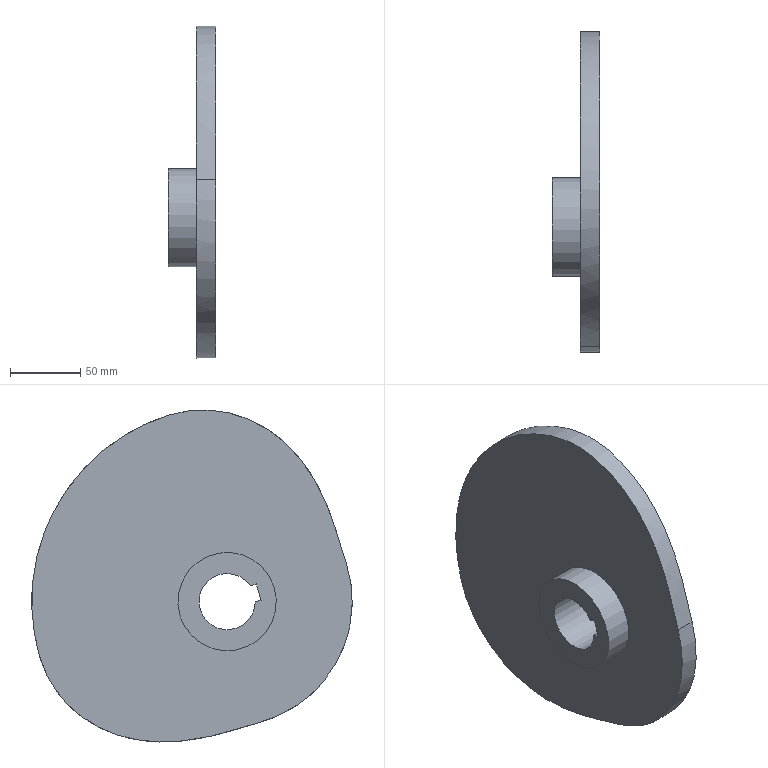Part | NX | features 100X000 2 | 1 solid | 10 faces | box 34 x 228.009 x 236.372 mm | volume 622668 mm3 | plane 6 | cylinder 2 | spline 2 | commonest cylinder face diameters 40 x1 70 x1
STEP:
#1=CARTESIAN_POINT('',(-103.5,-135.529,-808.87));
#2=VERTEX_POINT('',#1);
#3=CARTESIAN_POINT('',(-103.5,-138.999,-820.357));
#4=VERTEX_POINT('',#3);
#5=CARTESIAN_POINT('',(-103.5,-119.,-820.129));
#6=DIRECTION('',(-1.,0.,0.));
#7=DIRECTION('',(0.,0.9573,-0.2891));
#8=AXIS2_PLACEMENT_3D('',#5,#6,#7);
#9=CIRCLE('',#8,20.);
#10=EDGE_CURVE('',#2,#4,#9,.T.);
#11=ORIENTED_EDGE('',*,*,#10,.F.);
#12=CARTESIAN_POINT('',(-137.5,-135.529,-808.87));
#13=VERTEX_POINT('',#12);
#14=CARTESIAN_POINT('',(-103.5,-135.529,-808.87));
#15=DIRECTION('',(-1.,0.,0.));
#16=VECTOR('',#15,1000.);
#17=LINE('',#14,#16);
#18=EDGE_CURVE('',#2,#13,#17,.T.);
#19=ORIENTED_EDGE('',*,*,#18,.T.);
#20=CARTESIAN_POINT('',(-137.5,-138.999,-820.357));
#21=VERTEX_POINT('',#20);
#22=CARTESIAN_POINT('',(-137.5,-119.,-820.129));
#23=DIRECTION('',(1.,0.,0.));
#24=DIRECTION('',(0.,0.9573,-0.2891));
#25=AXIS2_PLACEMENT_3D('',#22,#23,#24);
#26=CIRCLE('',#25,20.);
#27=EDGE_CURVE('',#21,#13,#26,.T.);
#28=ORIENTED_EDGE('',*,*,#27,.F.);
#29=CARTESIAN_POINT('',(-137.5,-138.999,-820.357));
#30=DIRECTION('',(1.,0.,0.));
#31=VECTOR('',#30,1000.);
#32=LINE('',#29,#31);
#33=EDGE_CURVE('',#21,#4,#32,.T.);
#34=ORIENTED_EDGE('',*,*,#33,.T.);
#35=EDGE_LOOP('',(#11,#19,#28,#34));
#36=FACE_BOUND('',#35,.T.);
#37=CARTESIAN_POINT('',(218.943,-119.,-820.129));
#38=DIRECTION('',(-1.,0.,0.));
#39=DIRECTION('',(0.,0.9573,-0.2891));
#40=AXIS2_PLACEMENT_3D('',#37,#38,#39);
#41=CYLINDRICAL_SURFACE('',#40,20.);
#42=ADVANCED_FACE('',(#36),#41,.F.);
#43=CARTESIAN_POINT('',(-137.5,-143.231,-819.079));
#44=VERTEX_POINT('',#43);
#45=CARTESIAN_POINT('',(-137.5,-143.231,-819.079));
#46=DIRECTION('',(0.,0.9573,-0.2891));
#47=VECTOR('',#46,1000.);
#48=LINE('',#45,#47);
#49=EDGE_CURVE('',#44,#21,#48,.T.);
#50=ORIENTED_EDGE('',*,*,#49,.F.);
#51=CARTESIAN_POINT('',(-103.5,-143.231,-819.079));
#52=VERTEX_POINT('',#51);
#53=CARTESIAN_POINT('',(-137.5,-143.231,-819.079));
#54=DIRECTION('',(1.,0.,0.));
#55=VECTOR('',#54,1000.);
#56=LINE('',#53,#55);
#57=EDGE_CURVE('',#44,#52,#56,.T.);
#58=ORIENTED_EDGE('',*,*,#57,.T.);
#59=CARTESIAN_POINT('',(-103.5,-143.231,-819.079));
#60=DIRECTION('',(0.,0.9573,-0.2891));
#61=VECTOR('',#60,1000.);
#62=LINE('',#59,#61);
#63=EDGE_CURVE('',#52,#4,#62,.T.);
#64=ORIENTED_EDGE('',*,*,#63,.T.);
#65=ORIENTED_EDGE('',*,*,#33,.F.);
#66=EDGE_LOOP('',(#50,#58,#64,#65));
#67=FACE_BOUND('',#66,.T.);
#68=CARTESIAN_POINT('',(-103.5,-143.231,-819.079));
#69=DIRECTION('',(0.,-0.2891,-0.9573));
#70=DIRECTION('',(-1.,0.,0.));
#71=AXIS2_PLACEMENT_3D('',#68,#69,#70);
#72=PLANE('',#71);
#73=ADVANCED_FACE('',(#67),#72,.F.);
#74=CARTESIAN_POINT('',(-137.5,-139.762,-807.591));
#75=VERTEX_POINT('',#74);
#76=CARTESIAN_POINT('',(-137.5,-139.762,-807.591));
#77=DIRECTION('',(0.,-0.2891,-0.9573));
#78=VECTOR('',#77,1000.);
#79=LINE('',#76,#78);
#80=EDGE_CURVE('',#75,#44,#79,.T.);
#81=ORIENTED_EDGE('',*,*,#80,.F.);
#82=CARTESIAN_POINT('',(-103.5,-139.762,-807.591));
#83=VERTEX_POINT('',#82);
#84=CARTESIAN_POINT('',(-137.5,-139.762,-807.591));
#85=DIRECTION('',(1.,0.,0.));
#86=VECTOR('',#85,1000.);
#87=LINE('',#84,#86);
#88=EDGE_CURVE('',#75,#83,#87,.T.);
#89=ORIENTED_EDGE('',*,*,#88,.T.);
#90=CARTESIAN_POINT('',(-103.5,-139.762,-807.591));
#91=DIRECTION('',(0.,-0.2891,-0.9573));
#92=VECTOR('',#91,1000.);
#93=LINE('',#90,#92);
#94=EDGE_CURVE('',#83,#52,#93,.T.);
#95=ORIENTED_EDGE('',*,*,#94,.T.);
#96=ORIENTED_EDGE('',*,*,#57,.F.);
#97=EDGE_LOOP('',(#81,#89,#95,#96));
#98=FACE_BOUND('',#97,.T.);
#99=CARTESIAN_POINT('',(-103.5,-139.762,-807.591));
#100=DIRECTION('',(0.,-0.9573,0.2891));
#101=DIRECTION('',(-1.,0.,0.));
#102=AXIS2_PLACEMENT_3D('',#99,#100,#101);
#103=PLANE('',#102);
#104=ADVANCED_FACE('',(#98),#103,.F.);
#105=CARTESIAN_POINT('',(-117.5,-85.495,-830.249));
#106=VERTEX_POINT('',#105);
#107=CARTESIAN_POINT('',(-117.5,-119.,-820.129));
#108=DIRECTION('',(1.,0.,0.));
#109=DIRECTION('',(0.,0.9573,-0.2891));
#110=AXIS2_PLACEMENT_3D('',#107,#108,#109);
#111=CIRCLE('',#110,35.);
#112=EDGE_CURVE('',#106,#106,#111,.T.);
#113=ORIENTED_EDGE('',*,*,#112,.T.);
#114=EDGE_LOOP('',(#113));
#115=FACE_BOUND('',#114,.T.);
#116=CARTESIAN_POINT('',(-117.5,19.885,-825.794));
#117=VERTEX_POINT('',#116);
#118=CARTESIAN_POINT('',(-117.5,-203.83,-793.175));
#119=VERTEX_POINT('',#118);
#120=CARTESIAN_POINT('',(-117.5,-203.83,-793.175));
#121=CARTESIAN_POINT('',(-117.5,-206.1,-800.388));
#122=CARTESIAN_POINT('',(-117.5,-208.848,-815.383));
#123=CARTESIAN_POINT('',(-117.5,-207.135,-838.192));
#124=CARTESIAN_POINT('',(-117.5,-199.735,-859.831));
#125=CARTESIAN_POINT('',(-117.5,-187.117,-878.906));
#126=CARTESIAN_POINT('',(-117.5,-172.931,-891.635));
#127=CARTESIAN_POINT('',(-117.5,-159.935,-899.426));
#128=CARTESIAN_POINT('',(-117.5,-149.523,-903.996));
#129=CARTESIAN_POINT('',(-117.5,-138.618,-907.151));
#130=CARTESIAN_POINT('',(-117.5,-127.771,-910.449));
#131=CARTESIAN_POINT('',(-117.5,-116.863,-913.557));
#132=CARTESIAN_POINT('',(-117.5,-102.193,-917.232));
#133=CARTESIAN_POINT('',(-117.5,-83.496,-920.321));
#134=CARTESIAN_POINT('',(-117.5,-60.703,-920.128));
#135=CARTESIAN_POINT('',(-117.5,-38.429,-915.11));
#136=CARTESIAN_POINT('',(-117.5,-17.963,-904.903));
#137=CARTESIAN_POINT('',(-117.5,-0.8503,-889.705));
#138=CARTESIAN_POINT('',(-117.5,9.45,-873.606));
#139=CARTESIAN_POINT('',(-117.5,14.561,-859.339));
#140=CARTESIAN_POINT('',(-117.5,18.158,-844.637));
#141=CARTESIAN_POINT('',(-117.5,19.577,-833.35));
#142=CARTESIAN_POINT('',(-117.5,19.885,-825.794));
#143=B_SPLINE_CURVE_WITH_KNOTS('',3,(#120,#121,#122,#123,#124,#125,#126,#127,#128,#129,#130,#131,#132,#133,#134,#135,#136,#137,#138,#139,#140,#141,#142),.UNSPECIFIED.,.F.,.F.,(4,1,1,1,1,1,1,1,1,1,1,1,1,1,1,1,1,1,1,1,4),(0.,0.0625,0.125,0.1875,0.25,0.3125,0.3438,0.375,0.4062,0.4375,0.4688,0.5,0.5625,0.625,0.6875,0.75,0.8125,0.875,0.9062,0.9375,1.),.UNSPECIFIED.);
#144=EDGE_CURVE('',#117,#119,#143,.F.);
#145=ORIENTED_EDGE('',*,*,#144,.T.);
#146=CARTESIAN_POINT('',(-117.5,19.885,-825.794));
#147=CARTESIAN_POINT('',(-117.5,20.542,-810.441));
#148=CARTESIAN_POINT('',(-117.5,17.598,-787.258));
#149=CARTESIAN_POINT('',(-117.5,6.307,-758.571));
#150=CARTESIAN_POINT('',(-117.5,-5.545,-738.715));
#151=CARTESIAN_POINT('',(-117.5,-20.544,-721.111));
#152=CARTESIAN_POINT('',(-117.5,-38.233,-706.218));
#153=CARTESIAN_POINT('',(-117.5,-54.822,-696.403));
#154=CARTESIAN_POINT('',(-117.5,-68.935,-690.31));
#155=CARTESIAN_POINT('',(-117.5,-79.835,-686.529));
#156=CARTESIAN_POINT('',(-117.5,-91.128,-684.099));
#157=CARTESIAN_POINT('',(-117.5,-106.512,-683.184));
#158=CARTESIAN_POINT('',(-117.5,-125.675,-686.158));
#159=CARTESIAN_POINT('',(-117.5,-146.824,-695.82));
#160=CARTESIAN_POINT('',(-117.5,-164.847,-710.451));
#161=CARTESIAN_POINT('',(-117.5,-179.089,-728.734));
#162=CARTESIAN_POINT('',(-117.5,-189.587,-749.337));
#163=CARTESIAN_POINT('',(-117.5,-197.236,-771.098));
#164=CARTESIAN_POINT('',(-117.5,-201.598,-785.826));
#165=CARTESIAN_POINT('',(-117.5,-203.83,-793.175));
#166=B_SPLINE_CURVE_WITH_KNOTS('',3,(#146,#147,#148,#149,#150,#151,#152,#153,#154,#155,#156,#157,#158,#159,#160,#161,#162,#163,#164,#165),.UNSPECIFIED.,.F.,.F.,(4,1,1,1,1,1,1,1,1,1,1,1,1,1,1,1,1,4),(0.,0.125,0.1875,0.25,0.3125,0.375,0.4375,0.4688,0.5,0.5312,0.5625,0.625,0.6875,0.75,0.8125,0.875,0.9375,1.),.UNSPECIFIED.);
#167=EDGE_CURVE('',#119,#117,#166,.F.);
#168=ORIENTED_EDGE('',*,*,#167,.T.);
#169=EDGE_LOOP('',(#145,#168));
#170=FACE_BOUND('',#169,.T.);
#171=CARTESIAN_POINT('',(-117.5,-47.929,-928.307));
#172=DIRECTION('',(1.,0.,0.));
#173=DIRECTION('',(0.,-0.9573,0.2891));
#174=AXIS2_PLACEMENT_3D('',#171,#172,#173);
#175=PLANE('',#174);
#176=ADVANCED_FACE('',(#115,#170),#175,.F.);
#177=CARTESIAN_POINT('',(-103.5,-203.83,-793.175));
#178=VERTEX_POINT('',#177);
#179=CARTESIAN_POINT('',(-103.5,19.885,-825.794));
#180=VERTEX_POINT('',#179);
#181=CARTESIAN_POINT('',(-103.5,19.885,-825.794));
#182=CARTESIAN_POINT('',(-103.5,19.577,-833.349));
#183=CARTESIAN_POINT('',(-103.5,18.156,-844.636));
#184=CARTESIAN_POINT('',(-103.5,14.565,-859.339));
#185=CARTESIAN_POINT('',(-103.5,9.449,-873.606));
#186=CARTESIAN_POINT('',(-103.5,-0.8495,-889.704));
#187=CARTESIAN_POINT('',(-103.5,-17.962,-904.902));
#188=CARTESIAN_POINT('',(-103.5,-38.428,-915.11));
#189=CARTESIAN_POINT('',(-103.5,-60.702,-920.127));
#190=CARTESIAN_POINT('',(-103.5,-83.495,-920.321));
#191=CARTESIAN_POINT('',(-103.5,-102.191,-917.232));
#192=CARTESIAN_POINT('',(-103.5,-116.861,-913.557));
#193=CARTESIAN_POINT('',(-103.5,-127.77,-910.452));
#194=CARTESIAN_POINT('',(-103.5,-138.615,-907.15));
#195=CARTESIAN_POINT('',(-103.5,-149.521,-903.996));
#196=CARTESIAN_POINT('',(-103.5,-159.928,-899.413));
#197=CARTESIAN_POINT('',(-103.5,-172.931,-891.638));
#198=CARTESIAN_POINT('',(-103.5,-187.116,-878.904));
#199=CARTESIAN_POINT('',(-103.5,-199.733,-859.831));
#200=CARTESIAN_POINT('',(-103.5,-209.614,-830.978));
#201=CARTESIAN_POINT('',(-103.5,-208.416,-807.592));
#202=CARTESIAN_POINT('',(-103.5,-203.83,-793.175));
#203=B_SPLINE_CURVE_WITH_KNOTS('',3,(#181,#182,#183,#184,#185,#186,#187,#188,#189,#190,#191,#192,#193,#194,#195,#196,#197,#198,#199,#200,#201,#202),.UNSPECIFIED.,.F.,.F.,(4,1,1,1,1,1,1,1,1,1,1,1,1,1,1,1,1,1,1,4),(0.,0.0625,0.09375,0.125,0.1875,0.25,0.3125,0.375,0.4375,0.5,0.5312,0.5625,0.5938,0.625,0.6562,0.6875,0.75,0.8125,0.875,1.),.UNSPECIFIED.);
#204=EDGE_CURVE('',#178,#180,#203,.F.);
#205=ORIENTED_EDGE('',*,*,#204,.F.);
#206=CARTESIAN_POINT('',(-103.111,-203.83,-793.175));
#207=DIRECTION('',(-1.,0.,0.));
#208=VECTOR('',#207,1000.);
#209=LINE('',#206,#208);
#210=EDGE_CURVE('',#119,#178,#209,.F.);
#211=ORIENTED_EDGE('',*,*,#210,.F.);
#212=ORIENTED_EDGE('',*,*,#144,.F.);
#213=CARTESIAN_POINT('',(-103.111,19.885,-825.794));
#214=DIRECTION('',(-1.,0.,0.));
#215=VECTOR('',#214,1000.);
#216=LINE('',#213,#215);
#217=EDGE_CURVE('',#180,#117,#216,.T.);
#218=ORIENTED_EDGE('',*,*,#217,.F.);
#219=EDGE_LOOP('',(#205,#211,#212,#218));
#220=FACE_BOUND('',#219,.T.);
#221=CARTESIAN_POINT('',(-103.5,19.885,-825.794));
#222=CARTESIAN_POINT('',(-117.5,19.885,-825.794));
#223=CARTESIAN_POINT('',(-103.5,19.56,-833.741));
#224=CARTESIAN_POINT('',(-117.5,19.56,-833.741));
#225=CARTESIAN_POINT('',(-103.5,18.028,-845.325));
#226=CARTESIAN_POINT('',(-117.5,18.028,-845.325));
#227=CARTESIAN_POINT('',(-103.5,14.433,-859.739));
#228=CARTESIAN_POINT('',(-117.5,14.433,-859.739));
#229=CARTESIAN_POINT('',(-103.5,10.73,-869.978));
#230=CARTESIAN_POINT('',(-117.5,10.73,-869.978));
#231=CARTESIAN_POINT('',(-103.5,5.619,-879.516));
#232=CARTESIAN_POINT('',(-117.5,5.619,-879.516));
#233=CARTESIAN_POINT('',(-103.5,-0.8391,-888.445));
#234=CARTESIAN_POINT('',(-117.5,-0.8391,-888.445));
#235=CARTESIAN_POINT('',(-103.5,-8.305,-896.284));
#236=CARTESIAN_POINT('',(-117.5,-8.305,-896.284));
#237=CARTESIAN_POINT('',(-103.5,-16.795,-903.159));
#238=CARTESIAN_POINT('',(-117.5,-16.795,-903.159));
#239=CARTESIAN_POINT('',(-103.5,-26.109,-908.906));
#240=CARTESIAN_POINT('',(-117.5,-26.109,-908.906));
#241=CARTESIAN_POINT('',(-103.5,-35.953,-913.434));
#242=CARTESIAN_POINT('',(-117.5,-35.953,-913.434));
#243=CARTESIAN_POINT('',(-103.5,-46.394,-916.828));
#244=CARTESIAN_POINT('',(-117.5,-46.394,-916.828));
#245=CARTESIAN_POINT('',(-103.5,-57.036,-919.01));
#246=CARTESIAN_POINT('',(-117.5,-57.036,-919.01));
#247=CARTESIAN_POINT('',(-103.5,-67.843,-920.084));
#248=CARTESIAN_POINT('',(-117.5,-67.843,-920.084));
#249=CARTESIAN_POINT('',(-103.5,-82.467,-920.113));
#250=CARTESIAN_POINT('',(-117.5,-82.467,-920.113));
#251=CARTESIAN_POINT('',(-103.5,-96.728,-918.261));
#252=CARTESIAN_POINT('',(-117.5,-96.728,-918.261));
#253=CARTESIAN_POINT('',(-103.5,-110.806,-915.131));
#254=CARTESIAN_POINT('',(-117.5,-110.806,-915.131));
#255=CARTESIAN_POINT('',(-103.5,-121.295,-912.321));
#256=CARTESIAN_POINT('',(-117.5,-121.295,-912.321));
#257=CARTESIAN_POINT('',(-103.5,-131.724,-909.263));
#258=CARTESIAN_POINT('',(-117.5,-131.724,-909.263));
#259=CARTESIAN_POINT('',(-103.5,-140.397,-906.626));
#260=CARTESIAN_POINT('',(-117.5,-140.397,-906.626));
#261=CARTESIAN_POINT('',(-103.5,-147.324,-904.566));
#262=CARTESIAN_POINT('',(-117.5,-147.324,-904.566));
#263=CARTESIAN_POINT('',(-103.5,-154.26,-901.993));
#264=CARTESIAN_POINT('',(-117.5,-154.26,-901.993));
#265=CARTESIAN_POINT('',(-103.5,-162.89,-897.85));
#266=CARTESIAN_POINT('',(-117.5,-162.89,-897.85));
#267=CARTESIAN_POINT('',(-103.5,-172.887,-891.306));
#268=CARTESIAN_POINT('',(-117.5,-172.887,-891.306));
#269=CARTESIAN_POINT('',(-103.5,-185.273,-880.538));
#270=CARTESIAN_POINT('',(-117.5,-185.273,-880.538));
#271=CARTESIAN_POINT('',(-103.5,-198.112,-863.518));
#272=CARTESIAN_POINT('',(-117.5,-198.112,-863.518));
#273=CARTESIAN_POINT('',(-103.5,-207.077,-839.501));
#274=CARTESIAN_POINT('',(-117.5,-207.077,-839.501));
#275=CARTESIAN_POINT('',(-103.5,-208.585,-819.052));
#276=CARTESIAN_POINT('',(-117.5,-208.585,-819.052));
#277=CARTESIAN_POINT('',(-103.5,-206.738,-803.737));
#278=CARTESIAN_POINT('',(-117.5,-206.738,-803.737));
#279=CARTESIAN_POINT('',(-103.5,-204.877,-796.643));
#280=CARTESIAN_POINT('',(-117.5,-204.877,-796.643));
#281=CARTESIAN_POINT('',(-103.5,-203.83,-793.175));
#282=CARTESIAN_POINT('',(-117.5,-203.83,-793.175));
#283=B_SPLINE_SURFACE_WITH_KNOTS('',3,1,((#221,#222),(#223,#224),(#225,#226),(#227,#228),(#229,#230),(#231,#232),(#233,#234),(#235,#236),(#237,#238),(#239,#240),(#241,#242),(#243,#244),(#245,#246),(#247,#248),(#249,#250),(#251,#252),(#253,#254),(#255,#256),(#257,#258),(#259,#260),(#261,#262),(#263,#264),(#265,#266),(#267,#268),(#269,#270),(#271,#272),(#273,#274),(#275,#276),(#277,#278),(#279,#280),(#281,#282)),.SURF_OF_LINEAR_EXTRUSION.,.F.,.F.,.F.,(4,1,1,1,1,1,1,1,1,1,1,1,1,1,1,1,1,1,1,1,1,1,1,1,1,1,1,1,4),(2,2),(0.009286,0.07057,0.1012,0.1318,0.1625,0.1931,0.2238,0.2544,0.285,0.3157,0.3463,0.377,0.4076,0.4382,0.4995,0.5302,0.5608,0.5914,0.6221,0.6374,0.6527,0.6834,0.714,0.7446,0.8059,0.8672,0.9285,0.9591,0.9898),(0.,1.),.UNSPECIFIED.);
#284=ADVANCED_FACE('',(#220),#283,.T.);
#285=ORIENTED_EDGE('',*,*,#217,.T.);
#286=ORIENTED_EDGE('',*,*,#167,.F.);
#287=ORIENTED_EDGE('',*,*,#210,.T.);
#288=CARTESIAN_POINT('',(-103.5,-203.83,-793.175));
#289=CARTESIAN_POINT('',(-103.5,-201.598,-785.826));
#290=CARTESIAN_POINT('',(-103.5,-197.236,-771.098));
#291=CARTESIAN_POINT('',(-103.5,-189.587,-749.337));
#292=CARTESIAN_POINT('',(-103.5,-179.089,-728.734));
#293=CARTESIAN_POINT('',(-103.5,-164.848,-710.451));
#294=CARTESIAN_POINT('',(-103.5,-146.825,-695.82));
#295=CARTESIAN_POINT('',(-103.5,-125.676,-686.159));
#296=CARTESIAN_POINT('',(-103.5,-106.513,-683.184));
#297=CARTESIAN_POINT('',(-103.5,-91.128,-684.098));
#298=CARTESIAN_POINT('',(-103.5,-79.835,-686.528));
#299=CARTESIAN_POINT('',(-103.5,-68.935,-690.311));
#300=CARTESIAN_POINT('',(-103.5,-54.822,-696.403));
#301=CARTESIAN_POINT('',(-103.5,-38.232,-706.218));
#302=CARTESIAN_POINT('',(-103.5,-20.546,-721.115));
#303=CARTESIAN_POINT('',(-103.5,-5.543,-738.715));
#304=CARTESIAN_POINT('',(-103.5,6.304,-758.573));
#305=CARTESIAN_POINT('',(-103.5,17.599,-787.258));
#306=CARTESIAN_POINT('',(-103.5,20.543,-810.441));
#307=CARTESIAN_POINT('',(-103.5,19.885,-825.794));
#308=B_SPLINE_CURVE_WITH_KNOTS('',3,(#288,#289,#290,#291,#292,#293,#294,#295,#296,#297,#298,#299,#300,#301,#302,#303,#304,#305,#306,#307),.UNSPECIFIED.,.F.,.F.,(4,1,1,1,1,1,1,1,1,1,1,1,1,1,1,1,1,4),(0.,0.0625,0.125,0.1875,0.25,0.3125,0.375,0.4375,0.4688,0.5,0.5312,0.5625,0.625,0.6875,0.75,0.8125,0.875,1.),.UNSPECIFIED.);
#309=EDGE_CURVE('',#180,#178,#308,.F.);
#310=ORIENTED_EDGE('',*,*,#309,.F.);
#311=EDGE_LOOP('',(#285,#286,#287,#310));
#312=FACE_BOUND('',#311,.T.);
#313=CARTESIAN_POINT('',(-103.5,-203.83,-793.175));
#314=CARTESIAN_POINT('',(-117.5,-203.83,-793.175));
#315=CARTESIAN_POINT('',(-103.5,-201.737,-786.243));
#316=CARTESIAN_POINT('',(-117.5,-201.737,-786.243));
#317=CARTESIAN_POINT('',(-103.5,-197.598,-772.367));
#318=CARTESIAN_POINT('',(-117.5,-197.598,-772.367));
#319=CARTESIAN_POINT('',(-103.5,-190.539,-751.822));
#320=CARTESIAN_POINT('',(-117.5,-190.539,-751.822));
#321=CARTESIAN_POINT('',(-103.5,-182.644,-735.452));
#322=CARTESIAN_POINT('',(-117.5,-182.644,-735.452));
#323=CARTESIAN_POINT('',(-103.5,-174.811,-723.42));
#324=CARTESIAN_POINT('',(-117.5,-174.811,-723.42));
#325=CARTESIAN_POINT('',(-103.5,-168.061,-714.915));
#326=CARTESIAN_POINT('',(-117.5,-168.061,-714.915));
#327=CARTESIAN_POINT('',(-103.5,-160.402,-707.1));
#328=CARTESIAN_POINT('',(-117.5,-160.402,-707.1));
#329=CARTESIAN_POINT('',(-103.5,-149.296,-697.997));
#330=CARTESIAN_POINT('',(-117.5,-149.296,-697.997));
#331=CARTESIAN_POINT('',(-103.5,-136.458,-690.782));
#332=CARTESIAN_POINT('',(-117.5,-136.458,-690.782));
#333=CARTESIAN_POINT('',(-103.5,-122.872,-686.228));
#334=CARTESIAN_POINT('',(-117.5,-122.872,-686.228));
#335=CARTESIAN_POINT('',(-103.5,-112.174,-684.107));
#336=CARTESIAN_POINT('',(-117.5,-112.174,-684.107));
#337=CARTESIAN_POINT('',(-103.5,-101.27,-683.444));
#338=CARTESIAN_POINT('',(-117.5,-101.27,-683.444));
#339=CARTESIAN_POINT('',(-103.5,-90.523,-684.22));
#340=CARTESIAN_POINT('',(-117.5,-90.523,-684.22));
#341=CARTESIAN_POINT('',(-103.5,-79.82,-686.544));
#342=CARTESIAN_POINT('',(-117.5,-79.82,-686.544));
#343=CARTESIAN_POINT('',(-103.5,-65.876,-691.347));
#344=CARTESIAN_POINT('',(-117.5,-65.876,-691.347));
#345=CARTESIAN_POINT('',(-103.5,-48.323,-699.632));
#346=CARTESIAN_POINT('',(-117.5,-48.323,-699.632));
#347=CARTESIAN_POINT('',(-103.5,-28.382,-713.759));
#348=CARTESIAN_POINT('',(-117.5,-28.382,-713.759));
#349=CARTESIAN_POINT('',(-103.5,-10.666,-731.798));
#350=CARTESIAN_POINT('',(-117.5,-10.666,-731.798));
#351=CARTESIAN_POINT('',(-103.5,3.702,-753.151));
#352=CARTESIAN_POINT('',(-117.5,3.702,-753.151));
#353=CARTESIAN_POINT('',(-103.5,17.312,-784.698));
#354=CARTESIAN_POINT('',(-117.5,17.312,-784.698));
#355=CARTESIAN_POINT('',(-103.5,20.533,-809.9));
#356=CARTESIAN_POINT('',(-117.5,20.533,-809.9));
#357=CARTESIAN_POINT('',(-103.5,19.885,-825.794));
#358=CARTESIAN_POINT('',(-117.5,19.885,-825.794));
#359=B_SPLINE_SURFACE_WITH_KNOTS('',3,1,((#313,#314),(#315,#316),(#317,#318),(#319,#320),(#321,#322),(#323,#324),(#325,#326),(#327,#328),(#329,#330),(#331,#332),(#333,#334),(#335,#336),(#337,#338),(#339,#340),(#341,#342),(#343,#344),(#345,#346),(#347,#348),(#349,#350),(#351,#352),(#353,#354),(#355,#356),(#357,#358)),.SURF_OF_LINEAR_EXTRUSION.,.F.,.F.,.F.,(4,1,1,1,1,1,1,1,1,1,1,1,1,1,1,1,1,1,1,1,4),(2,2),(0.0104,0.07166,0.1329,0.1942,0.2248,0.2554,0.2861,0.3167,0.378,0.4086,0.4392,0.4699,0.5005,0.5311,0.5617,0.623,0.6843,0.7455,0.8068,0.868,0.9906),(0.,1.),.UNSPECIFIED.);
#360=ADVANCED_FACE('',(#312),#359,.T.);
#361=CARTESIAN_POINT('',(-103.5,-135.529,-808.87));
#362=DIRECTION('',(0.,-0.9573,0.2891));
#363=VECTOR('',#362,1000.);
#364=LINE('',#361,#363);
#365=EDGE_CURVE('',#2,#83,#364,.T.);
#366=ORIENTED_EDGE('',*,*,#365,.F.);
#367=ORIENTED_EDGE('',*,*,#10,.T.);
#368=ORIENTED_EDGE('',*,*,#63,.F.);
#369=ORIENTED_EDGE('',*,*,#94,.F.);
#370=EDGE_LOOP('',(#366,#367,#368,#369));
#371=FACE_BOUND('',#370,.T.);
#372=ORIENTED_EDGE('',*,*,#204,.T.);
#373=ORIENTED_EDGE('',*,*,#309,.T.);
#374=EDGE_LOOP('',(#372,#373));
#375=FACE_BOUND('',#374,.T.);
#376=CARTESIAN_POINT('',(-103.5,-47.929,-928.307));
#377=DIRECTION('',(1.,0.,0.));
#378=DIRECTION('',(0.,-0.9573,0.2891));
#379=AXIS2_PLACEMENT_3D('',#376,#377,#378);
#380=PLANE('',#379);
#381=ADVANCED_FACE('',(#371,#375),#380,.T.);
#382=ORIENTED_EDGE('',*,*,#88,.F.);
#383=CARTESIAN_POINT('',(-137.5,-135.529,-808.87));
#384=DIRECTION('',(0.,-0.9573,0.2891));
#385=VECTOR('',#384,1000.);
#386=LINE('',#383,#385);
#387=EDGE_CURVE('',#13,#75,#386,.T.);
#388=ORIENTED_EDGE('',*,*,#387,.F.);
#389=ORIENTED_EDGE('',*,*,#18,.F.);
#390=ORIENTED_EDGE('',*,*,#365,.T.);
#391=EDGE_LOOP('',(#382,#388,#389,#390));
#392=FACE_BOUND('',#391,.T.);
#393=CARTESIAN_POINT('',(-103.5,-139.762,-807.591));
#394=DIRECTION('',(0.,0.2891,0.9573));
#395=DIRECTION('',(1.,0.,0.));
#396=AXIS2_PLACEMENT_3D('',#393,#394,#395);
#397=PLANE('',#396);
#398=ADVANCED_FACE('',(#392),#397,.F.);
#399=ORIENTED_EDGE('',*,*,#80,.T.);
#400=ORIENTED_EDGE('',*,*,#49,.T.);
#401=ORIENTED_EDGE('',*,*,#27,.T.);
#402=ORIENTED_EDGE('',*,*,#387,.T.);
#403=EDGE_LOOP('',(#399,#400,#401,#402));
#404=FACE_BOUND('',#403,.T.);
#405=CARTESIAN_POINT('',(-137.5,-152.505,-810.01));
#406=VERTEX_POINT('',#405);
#407=CARTESIAN_POINT('',(-137.5,-119.,-820.129));
#408=DIRECTION('',(-1.,0.,0.));
#409=DIRECTION('',(0.,-0.9573,0.2891));
#410=AXIS2_PLACEMENT_3D('',#407,#408,#409);
#411=CIRCLE('',#410,35.);
#412=EDGE_CURVE('',#406,#406,#411,.T.);
#413=ORIENTED_EDGE('',*,*,#412,.T.);
#414=EDGE_LOOP('',(#413));
#415=FACE_BOUND('',#414,.T.);
#416=CARTESIAN_POINT('',(-137.5,-119.,-820.129));
#417=DIRECTION('',(-1.,0.,0.));
#418=DIRECTION('',(0.,0.9573,-0.2891));
#419=AXIS2_PLACEMENT_3D('',#416,#417,#418);
#420=PLANE('',#419);
#421=ADVANCED_FACE('',(#404,#415),#420,.T.);
#422=ORIENTED_EDGE('',*,*,#412,.F.);
#423=EDGE_LOOP('',(#422));
#424=FACE_BOUND('',#423,.T.);
#425=ORIENTED_EDGE('',*,*,#112,.F.);
#426=EDGE_LOOP('',(#425));
#427=FACE_BOUND('',#426,.T.);
#428=CARTESIAN_POINT('',(-137.5,-119.,-820.129));
#429=DIRECTION('',(1.,0.,0.));
#430=DIRECTION('',(0.,-0.9573,0.2891));
#431=AXIS2_PLACEMENT_3D('',#428,#429,#430);
#432=CYLINDRICAL_SURFACE('',#431,35.);
#433=ADVANCED_FACE('',(#424,#427),#432,.T.);
#434=CLOSED_SHELL('',(#42,#73,#104,#176,#284,#360,#381,#398,#421,#433));
#435=MANIFOLD_SOLID_BREP('',#434);
#436=(LENGTH_UNIT()NAMED_UNIT(*)SI_UNIT(.MILLI.,.METRE.));
#437=UNCERTAINTY_MEASURE_WITH_UNIT(LENGTH_MEASURE(0.0508),#436,'','');
#438=(NAMED_UNIT(*)PLANE_ANGLE_UNIT()SI_UNIT($,.RADIAN.));
#439=(NAMED_UNIT(*)SI_UNIT($,.STERADIAN.)SOLID_ANGLE_UNIT());
#440=(GEOMETRIC_REPRESENTATION_CONTEXT(3)GLOBAL_UNCERTAINTY_ASSIGNED_CONTEXT((#437))GLOBAL_UNIT_ASSIGNED_CONTEXT((#436,#438,#439))REPRESENTATION_CONTEXT('',''));
#441=ADVANCED_BREP_SHAPE_REPRESENTATION('',(#435),#440);